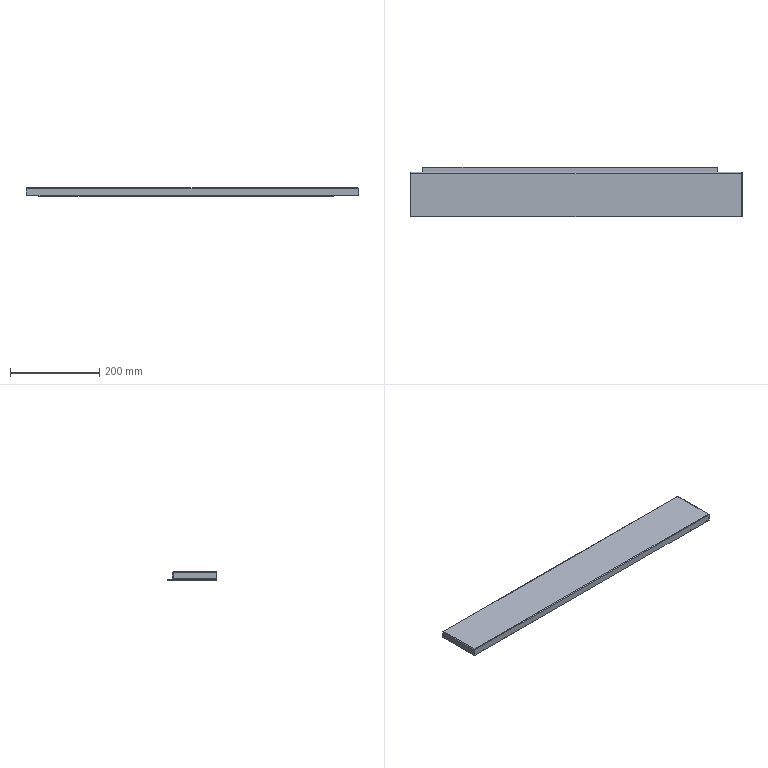Part | NX | features BREP 3 | 3 solids | 86 faces | box 745 x 112 x 18 mm | volume 171953 mm3 | plane 72 | cylinder 14 | commonest cylinder face diameters 0.02 x7 3.02 x7